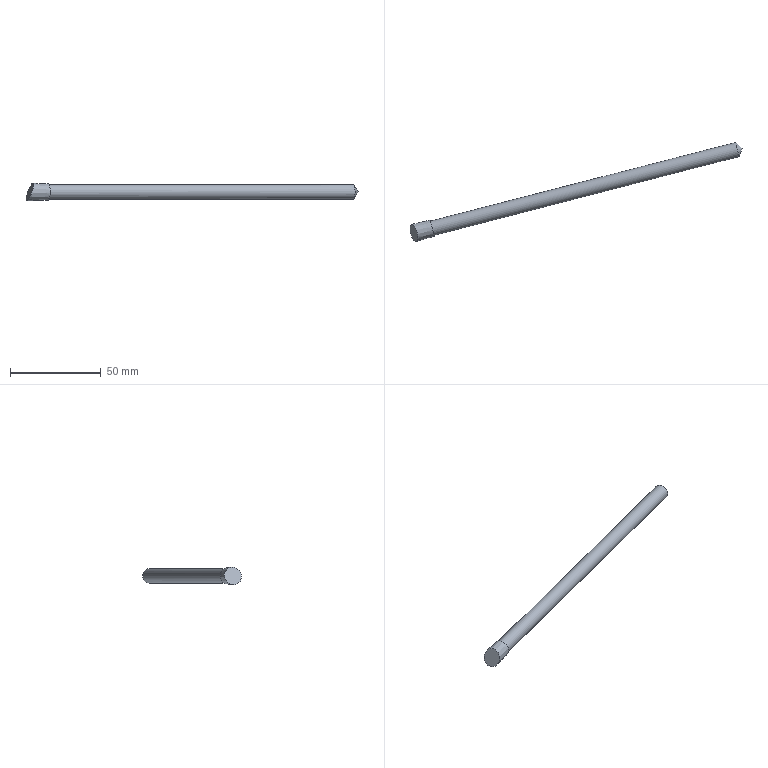Part | STEP file | 车灯-后视镜_id34_x_t | 1 solid | 5 faces | box 182.446 x 54.425 x 9.706 mm | volume 9470 mm3 | plane 2 | cone 2 | cylinder 1 | commonest cylinder face diameters 8 x1
STEP:
#1=CARTESIAN_POINT('',(-174.996,8.011,43.714));
#2=VERTEX_POINT('',#1);
#3=CARTESIAN_POINT('',(-173.997,4.138,43.714));
#4=DIRECTION('',(-0.9683,-0.2497,0.));
#5=DIRECTION('',(-0.2497,0.9683,0.));
#6=AXIS2_PLACEMENT_3D('',#3,#4,#5);
#7=CIRCLE('',#6,4.);
#8=EDGE_CURVE('',#2,#2,#7,.T.);
#9=ORIENTED_EDGE('',*,*,#8,.T.);
#10=EDGE_LOOP('',(#9));
#11=FACE_BOUND('',#10,.T.);
#12=CARTESIAN_POINT('',(-173.997,4.138,39.179));
#13=VERTEX_POINT('',#12);
#14=CARTESIAN_POINT('',(-173.997,4.138,43.714));
#15=DIRECTION('',(0.9683,0.2497,0.));
#16=DIRECTION('',(0.,0.,-1.));
#17=AXIS2_PLACEMENT_3D('',#14,#15,#16);
#18=CIRCLE('',#17,4.535);
#19=EDGE_CURVE('',#13,#13,#18,.T.);
#20=ORIENTED_EDGE('',*,*,#19,.T.);
#21=EDGE_LOOP('',(#20));
#22=FACE_BOUND('',#21,.T.);
#23=CARTESIAN_POINT('',(-173.997,4.138,43.714));
#24=DIRECTION('',(0.9683,0.2497,0.));
#25=DIRECTION('',(0.,0.,1.));
#26=AXIS2_PLACEMENT_3D('',#23,#24,#25);
#27=PLANE('',#26);
#28=ADVANCED_FACE('',(#11,#22),#27,.T.);
#29=CARTESIAN_POINT('',(-185.847,1.082,38.808));
#30=VERTEX_POINT('',#29);
#31=CARTESIAN_POINT('',(-184.137,1.523,43.661));
#32=DIRECTION('',(-0.9099,-0.2346,0.342));
#33=DIRECTION('',(-0.3312,-0.0854,-0.9397));
#34=AXIS2_PLACEMENT_3D('',#31,#32,#33);
#35=ELLIPSE('',#34,5.164,4.852);
#36=EDGE_CURVE('',#30,#30,#35,.T.);
#37=ORIENTED_EDGE('',*,*,#36,.F.);
#38=EDGE_LOOP('',(#37));
#39=FACE_BOUND('',#38,.T.);
#40=ORIENTED_EDGE('',*,*,#19,.F.);
#41=EDGE_LOOP('',(#40));
#42=FACE_BOUND('',#41,.T.);
#43=CARTESIAN_POINT('',(-173.997,4.138,43.714));
#44=DIRECTION('',(-0.9683,-0.2497,0.));
#45=DIRECTION('',(0.,0.,-1.));
#46=AXIS2_PLACEMENT_3D('',#43,#44,#45);
#47=CONICAL_SURFACE('',#46,4.535,1.738);
#48=ADVANCED_FACE('',(#39,#42),#47,.T.);
#49=ORIENTED_EDGE('',*,*,#8,.F.);
#50=EDGE_LOOP('',(#49));
#51=FACE_BOUND('',#50,.T.);
#52=CARTESIAN_POINT('',(-6.4,47.356,39.714));
#53=VERTEX_POINT('',#52);
#54=CARTESIAN_POINT('',(-6.4,47.356,43.714));
#55=DIRECTION('',(0.9683,0.2497,0.));
#56=DIRECTION('',(0.,0.,-1.));
#57=AXIS2_PLACEMENT_3D('',#54,#55,#56);
#58=CIRCLE('',#57,4.);
#59=EDGE_CURVE('',#53,#53,#58,.T.);
#60=ORIENTED_EDGE('',*,*,#59,.F.);
#61=EDGE_LOOP('',(#60));
#62=FACE_BOUND('',#61,.T.);
#63=CARTESIAN_POINT('',(-127.44,16.144,43.714));
#64=DIRECTION('',(0.9683,0.2497,0.));
#65=DIRECTION('',(0.,0.,1.));
#66=AXIS2_PLACEMENT_3D('',#63,#64,#65);
#67=CYLINDRICAL_SURFACE('',#66,4.);
#68=ADVANCED_FACE('',(#51,#62),#67,.T.);
#69=ORIENTED_EDGE('',*,*,#59,.T.);
#70=EDGE_LOOP('',(#69));
#71=FACE_BOUND('',#70,.T.);
#72=CARTESIAN_POINT('',(-3.787,48.03,43.714));
#73=VERTEX_POINT('',#72);
#74=VERTEX_LOOP('',#73);
#75=FACE_BOUND('',#74,.T.);
#76=CARTESIAN_POINT('',(-3.787,48.03,43.714));
#77=DIRECTION('',(-0.9683,-0.2497,0.));
#78=DIRECTION('',(0.,0.,1.));
#79=AXIS2_PLACEMENT_3D('',#76,#77,#78);
#80=CONICAL_SURFACE('',#79,0.,56.);
#81=ADVANCED_FACE('',(#71,#75),#80,.T.);
#82=ORIENTED_EDGE('',*,*,#36,.T.);
#83=EDGE_LOOP('',(#82));
#84=FACE_OUTER_BOUND('',#83,.T.);
#85=CARTESIAN_POINT('',(-192.021,21.97,36.714));
#86=DIRECTION('',(-0.9099,-0.2346,0.342));
#87=DIRECTION('',(0.3518,0.,0.9361));
#88=AXIS2_PLACEMENT_3D('',#85,#86,#87);
#89=PLANE('',#88);
#90=ADVANCED_FACE('',(#84),#89,.T.);
#91=CLOSED_SHELL('',(#28,#48,#68,#81,#90));
#92=MANIFOLD_SOLID_BREP('',#91);
#93=(LENGTH_UNIT()NAMED_UNIT(*)SI_UNIT(.MILLI.,.METRE.));
#94=UNCERTAINTY_MEASURE_WITH_UNIT(LENGTH_MEASURE(0.00002),#93,'','');
#95=(NAMED_UNIT(*)PLANE_ANGLE_UNIT()SI_UNIT($,.RADIAN.));
#96=PLANE_ANGLE_MEASURE_WITH_UNIT(PLANE_ANGLE_MEASURE(0.01745),#95);
#97=DIMENSIONAL_EXPONENTS(0.,0.,0.,0.,0.,0.,0.);
#98=(CONVERSION_BASED_UNIT('DEGREE',#96)NAMED_UNIT(#97)PLANE_ANGLE_UNIT());
#99=(NAMED_UNIT(*)SI_UNIT($,.STERADIAN.)SOLID_ANGLE_UNIT());
#100=(GEOMETRIC_REPRESENTATION_CONTEXT(3)GLOBAL_UNCERTAINTY_ASSIGNED_CONTEXT((#94))GLOBAL_UNIT_ASSIGNED_CONTEXT((#93,#98,#99))REPRESENTATION_CONTEXT('',''));
#101=ADVANCED_BREP_SHAPE_REPRESENTATION('',(#92),#100);